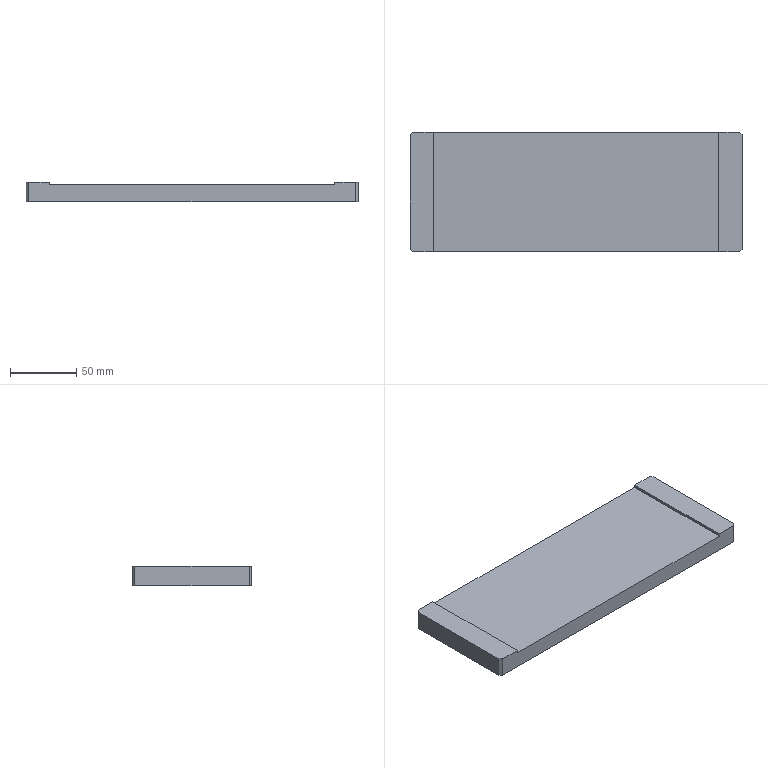Part | STEP file | 001-003-Shaft storage slider connecting plate | 1 solid | 14 faces | box 250 x 90 x 15 mm | volume 298680 mm3 | plane 14
STEP:
#1=CARTESIAN_POINT('',(0.,0.,0.));
#2=DIRECTION('',(0.,0.,1.));
#3=DIRECTION('',(1.,0.,0.));
#4=AXIS2_PLACEMENT_3D('',#1,#2,#3);
#5=CARTESIAN_POINT('',(123.,45.,15.));
#6=VERTEX_POINT('',#5);
#7=CARTESIAN_POINT('',(107.5,45.,15.));
#8=VERTEX_POINT('',#7);
#9=CARTESIAN_POINT('',(-125.,45.,15.));
#10=DIRECTION('',(-1.,0.,0.));
#11=VECTOR('',#10,1.);
#12=LINE('',#9,#11);
#13=CARTESIAN_POINT('',(0.,0.,15.));
#14=DIRECTION('',(0.,0.,-1.));
#15=DIRECTION('',(-1.,0.,0.));
#16=AXIS2_PLACEMENT_3D('',#13,#14,#15);
#17=PLANE('',#16);
#18=CARTESIAN_POINT('',(125.,45.));
#19=DIRECTION('',(1.,0.));
#20=VECTOR('',#19,1.);
#21=LINE('',#18,#20);
#22=(GEOMETRIC_REPRESENTATION_CONTEXT(2)PARAMETRIC_REPRESENTATION_CONTEXT()REPRESENTATION_CONTEXT('',''));
#23=DEFINITIONAL_REPRESENTATION('',(#21),#22);
#24=PCURVE('',#17,#23);
#25=CARTESIAN_POINT('',(-125.,45.,15.));
#26=DIRECTION('',(0.,-1.,0.));
#27=DIRECTION('',(0.,0.,-1.));
#28=AXIS2_PLACEMENT_3D('',#25,#26,#27);
#29=PLANE('',#28);
#30=CARTESIAN_POINT('',(0.,0.));
#31=DIRECTION('',(0.,-1.));
#32=VECTOR('',#31,1.);
#33=LINE('',#30,#32);
#34=(GEOMETRIC_REPRESENTATION_CONTEXT(2)PARAMETRIC_REPRESENTATION_CONTEXT()REPRESENTATION_CONTEXT('',''));
#35=DEFINITIONAL_REPRESENTATION('',(#33),#34);
#36=PCURVE('',#29,#35);
#37=SURFACE_CURVE('',#12,(#24,#36),.PCURVE_S1.);
#38=EDGE_CURVE('',#6,#8,#37,.T.);
#39=ORIENTED_EDGE('',*,*,#38,.T.);
#40=CARTESIAN_POINT('',(107.5,-45.,15.));
#41=VERTEX_POINT('',#40);
#42=CARTESIAN_POINT('',(107.5,-45.,15.));
#43=DIRECTION('',(0.,1.,0.));
#44=VECTOR('',#43,1.);
#45=LINE('',#42,#44);
#46=CARTESIAN_POINT('',(-107.5,-45.));
#47=DIRECTION('',(0.,1.));
#48=VECTOR('',#47,1.);
#49=LINE('',#46,#48);
#50=(GEOMETRIC_REPRESENTATION_CONTEXT(2)PARAMETRIC_REPRESENTATION_CONTEXT()REPRESENTATION_CONTEXT('',''));
#51=DEFINITIONAL_REPRESENTATION('',(#49),#50);
#52=PCURVE('',#17,#51);
#53=CARTESIAN_POINT('',(107.5,-45.,15.));
#54=DIRECTION('',(1.,0.,0.));
#55=DIRECTION('',(0.,0.,-1.));
#56=AXIS2_PLACEMENT_3D('',#53,#54,#55);
#57=PLANE('',#56);
#58=CARTESIAN_POINT('',(0.,0.));
#59=DIRECTION('',(0.,1.));
#60=VECTOR('',#59,1.);
#61=LINE('',#58,#60);
#62=(GEOMETRIC_REPRESENTATION_CONTEXT(2)PARAMETRIC_REPRESENTATION_CONTEXT()REPRESENTATION_CONTEXT('',''));
#63=DEFINITIONAL_REPRESENTATION('',(#61),#62);
#64=PCURVE('',#57,#63);
#65=SURFACE_CURVE('',#45,(#52,#64),.PCURVE_S1.);
#66=EDGE_CURVE('',#41,#8,#65,.T.);
#67=ORIENTED_EDGE('',*,*,#66,.F.);
#68=CARTESIAN_POINT('',(123.,-45.,15.));
#69=VERTEX_POINT('',#68);
#70=CARTESIAN_POINT('',(-125.,-45.,15.));
#71=DIRECTION('',(1.,0.,0.));
#72=VECTOR('',#71,1.);
#73=LINE('',#70,#72);
#74=CARTESIAN_POINT('',(125.,-45.));
#75=DIRECTION('',(-1.,0.));
#76=VECTOR('',#75,1.);
#77=LINE('',#74,#76);
#78=(GEOMETRIC_REPRESENTATION_CONTEXT(2)PARAMETRIC_REPRESENTATION_CONTEXT()REPRESENTATION_CONTEXT('',''));
#79=DEFINITIONAL_REPRESENTATION('',(#77),#78);
#80=PCURVE('',#17,#79);
#81=CARTESIAN_POINT('',(-125.,-45.,15.));
#82=DIRECTION('',(0.,1.,0.));
#83=DIRECTION('',(0.,0.,1.));
#84=AXIS2_PLACEMENT_3D('',#81,#82,#83);
#85=PLANE('',#84);
#86=CARTESIAN_POINT('',(0.,0.));
#87=DIRECTION('',(0.,1.));
#88=VECTOR('',#87,1.);
#89=LINE('',#86,#88);
#90=(GEOMETRIC_REPRESENTATION_CONTEXT(2)PARAMETRIC_REPRESENTATION_CONTEXT()REPRESENTATION_CONTEXT('',''));
#91=DEFINITIONAL_REPRESENTATION('',(#89),#90);
#92=PCURVE('',#85,#91);
#93=SURFACE_CURVE('',#73,(#80,#92),.PCURVE_S1.);
#94=EDGE_CURVE('',#41,#69,#93,.T.);
#95=ORIENTED_EDGE('',*,*,#94,.T.);
#96=CARTESIAN_POINT('',(125.,-43.,15.));
#97=VERTEX_POINT('',#96);
#98=CARTESIAN_POINT('',(125.,-43.,15.));
#99=DIRECTION('',(0.7071,0.7071,0.));
#100=VECTOR('',#99,1.);
#101=LINE('',#98,#100);
#102=CARTESIAN_POINT('',(-125.,-43.));
#103=DIRECTION('',(-0.7071,0.7071));
#104=VECTOR('',#103,1.);
#105=LINE('',#102,#104);
#106=(GEOMETRIC_REPRESENTATION_CONTEXT(2)PARAMETRIC_REPRESENTATION_CONTEXT()REPRESENTATION_CONTEXT('',''));
#107=DEFINITIONAL_REPRESENTATION('',(#105),#106);
#108=PCURVE('',#17,#107);
#109=CARTESIAN_POINT('',(125.,-43.,15.));
#110=DIRECTION('',(-0.7071,0.7071,0.));
#111=DIRECTION('',(0.,0.,-1.));
#112=AXIS2_PLACEMENT_3D('',#109,#110,#111);
#113=PLANE('',#112);
#114=CARTESIAN_POINT('',(0.,0.));
#115=DIRECTION('',(0.,-1.));
#116=VECTOR('',#115,1.);
#117=LINE('',#114,#116);
#118=(GEOMETRIC_REPRESENTATION_CONTEXT(2)PARAMETRIC_REPRESENTATION_CONTEXT()REPRESENTATION_CONTEXT('',''));
#119=DEFINITIONAL_REPRESENTATION('',(#117),#118);
#120=PCURVE('',#113,#119);
#121=SURFACE_CURVE('',#101,(#108,#120),.PCURVE_S1.);
#122=EDGE_CURVE('',#69,#97,#121,.T.);
#123=ORIENTED_EDGE('',*,*,#122,.T.);
#124=CARTESIAN_POINT('',(125.,43.,15.));
#125=VERTEX_POINT('',#124);
#126=CARTESIAN_POINT('',(125.,-45.,15.));
#127=DIRECTION('',(0.,1.,0.));
#128=VECTOR('',#127,1.);
#129=LINE('',#126,#128);
#130=CARTESIAN_POINT('',(-125.,-45.));
#131=DIRECTION('',(0.,1.));
#132=VECTOR('',#131,1.);
#133=LINE('',#130,#132);
#134=(GEOMETRIC_REPRESENTATION_CONTEXT(2)PARAMETRIC_REPRESENTATION_CONTEXT()REPRESENTATION_CONTEXT('',''));
#135=DEFINITIONAL_REPRESENTATION('',(#133),#134);
#136=PCURVE('',#17,#135);
#137=CARTESIAN_POINT('',(125.,-45.,15.));
#138=DIRECTION('',(-1.,0.,0.));
#139=DIRECTION('',(0.,0.,1.));
#140=AXIS2_PLACEMENT_3D('',#137,#138,#139);
#141=PLANE('',#140);
#142=CARTESIAN_POINT('',(0.,0.));
#143=DIRECTION('',(0.,1.));
#144=VECTOR('',#143,1.);
#145=LINE('',#142,#144);
#146=(GEOMETRIC_REPRESENTATION_CONTEXT(2)PARAMETRIC_REPRESENTATION_CONTEXT()REPRESENTATION_CONTEXT('',''));
#147=DEFINITIONAL_REPRESENTATION('',(#145),#146);
#148=PCURVE('',#141,#147);
#149=SURFACE_CURVE('',#129,(#136,#148),.PCURVE_S1.);
#150=EDGE_CURVE('',#97,#125,#149,.T.);
#151=ORIENTED_EDGE('',*,*,#150,.T.);
#152=CARTESIAN_POINT('',(123.,45.,15.));
#153=DIRECTION('',(-0.7071,0.7071,0.));
#154=VECTOR('',#153,1.);
#155=LINE('',#152,#154);
#156=CARTESIAN_POINT('',(-123.,45.));
#157=DIRECTION('',(0.7071,0.7071));
#158=VECTOR('',#157,1.);
#159=LINE('',#156,#158);
#160=(GEOMETRIC_REPRESENTATION_CONTEXT(2)PARAMETRIC_REPRESENTATION_CONTEXT()REPRESENTATION_CONTEXT('',''));
#161=DEFINITIONAL_REPRESENTATION('',(#159),#160);
#162=PCURVE('',#17,#161);
#163=CARTESIAN_POINT('',(123.,45.,15.));
#164=DIRECTION('',(-0.7071,-0.7071,0.));
#165=DIRECTION('',(0.,0.,-1.));
#166=AXIS2_PLACEMENT_3D('',#163,#164,#165);
#167=PLANE('',#166);
#168=CARTESIAN_POINT('',(0.,0.));
#169=DIRECTION('',(0.,-1.));
#170=VECTOR('',#169,1.);
#171=LINE('',#168,#170);
#172=(GEOMETRIC_REPRESENTATION_CONTEXT(2)PARAMETRIC_REPRESENTATION_CONTEXT()REPRESENTATION_CONTEXT('',''));
#173=DEFINITIONAL_REPRESENTATION('',(#171),#172);
#174=PCURVE('',#167,#173);
#175=SURFACE_CURVE('',#155,(#162,#174),.PCURVE_S1.);
#176=EDGE_CURVE('',#125,#6,#175,.T.);
#177=ORIENTED_EDGE('',*,*,#176,.T.);
#178=EDGE_LOOP('',(#39,#67,#95,#123,#151,#177));
#179=FACE_BOUND('',#178,.T.);
#180=ADVANCED_FACE('',(#179),#17,.F.);
#181=ORIENTED_EDGE('',*,*,#150,.F.);
#182=CARTESIAN_POINT('',(125.,-43.,0.));
#183=VERTEX_POINT('',#182);
#184=CARTESIAN_POINT('',(125.,-43.,15.));
#185=DIRECTION('',(0.,0.,-1.));
#186=VECTOR('',#185,1.);
#187=LINE('',#184,#186);
#188=CARTESIAN_POINT('',(0.,2.));
#189=DIRECTION('',(-1.,0.));
#190=VECTOR('',#189,1.);
#191=LINE('',#188,#190);
#192=(GEOMETRIC_REPRESENTATION_CONTEXT(2)PARAMETRIC_REPRESENTATION_CONTEXT()REPRESENTATION_CONTEXT('',''));
#193=DEFINITIONAL_REPRESENTATION('',(#191),#192);
#194=PCURVE('',#141,#193);
#195=CARTESIAN_POINT('',(0.,0.));
#196=DIRECTION('',(1.,0.));
#197=VECTOR('',#196,1.);
#198=LINE('',#195,#197);
#199=(GEOMETRIC_REPRESENTATION_CONTEXT(2)PARAMETRIC_REPRESENTATION_CONTEXT()REPRESENTATION_CONTEXT('',''));
#200=DEFINITIONAL_REPRESENTATION('',(#198),#199);
#201=PCURVE('',#113,#200);
#202=SURFACE_CURVE('',#187,(#194,#201),.PCURVE_S1.);
#203=EDGE_CURVE('',#97,#183,#202,.T.);
#204=ORIENTED_EDGE('',*,*,#203,.T.);
#205=CARTESIAN_POINT('',(125.,43.,0.));
#206=VERTEX_POINT('',#205);
#207=CARTESIAN_POINT('',(125.,-45.,0.));
#208=DIRECTION('',(0.,1.,0.));
#209=VECTOR('',#208,1.);
#210=LINE('',#207,#209);
#211=CARTESIAN_POINT('',(-15.,0.));
#212=DIRECTION('',(0.,1.));
#213=VECTOR('',#212,1.);
#214=LINE('',#211,#213);
#215=(GEOMETRIC_REPRESENTATION_CONTEXT(2)PARAMETRIC_REPRESENTATION_CONTEXT()REPRESENTATION_CONTEXT('',''));
#216=DEFINITIONAL_REPRESENTATION('',(#214),#215);
#217=PCURVE('',#141,#216);
#218=CARTESIAN_POINT('',(0.,0.,0.));
#219=DIRECTION('',(0.,0.,-1.));
#220=DIRECTION('',(-1.,0.,0.));
#221=AXIS2_PLACEMENT_3D('',#218,#219,#220);
#222=PLANE('',#221);
#223=CARTESIAN_POINT('',(-125.,-45.));
#224=DIRECTION('',(0.,1.));
#225=VECTOR('',#224,1.);
#226=LINE('',#223,#225);
#227=(GEOMETRIC_REPRESENTATION_CONTEXT(2)PARAMETRIC_REPRESENTATION_CONTEXT()REPRESENTATION_CONTEXT('',''));
#228=DEFINITIONAL_REPRESENTATION('',(#226),#227);
#229=PCURVE('',#222,#228);
#230=SURFACE_CURVE('',#210,(#217,#229),.PCURVE_S1.);
#231=EDGE_CURVE('',#183,#206,#230,.T.);
#232=ORIENTED_EDGE('',*,*,#231,.T.);
#233=CARTESIAN_POINT('',(125.,43.,15.));
#234=DIRECTION('',(0.,0.,1.));
#235=VECTOR('',#234,1.);
#236=LINE('',#233,#235);
#237=CARTESIAN_POINT('',(0.,88.));
#238=DIRECTION('',(1.,0.));
#239=VECTOR('',#238,1.);
#240=LINE('',#237,#239);
#241=(GEOMETRIC_REPRESENTATION_CONTEXT(2)PARAMETRIC_REPRESENTATION_CONTEXT()REPRESENTATION_CONTEXT('',''));
#242=DEFINITIONAL_REPRESENTATION('',(#240),#241);
#243=PCURVE('',#141,#242);
#244=CARTESIAN_POINT('',(0.,2.828));
#245=DIRECTION('',(-1.,0.));
#246=VECTOR('',#245,1.);
#247=LINE('',#244,#246);
#248=(GEOMETRIC_REPRESENTATION_CONTEXT(2)PARAMETRIC_REPRESENTATION_CONTEXT()REPRESENTATION_CONTEXT('',''));
#249=DEFINITIONAL_REPRESENTATION('',(#247),#248);
#250=PCURVE('',#167,#249);
#251=SURFACE_CURVE('',#236,(#243,#250),.PCURVE_S1.);
#252=EDGE_CURVE('',#206,#125,#251,.T.);
#253=ORIENTED_EDGE('',*,*,#252,.T.);
#254=EDGE_LOOP('',(#181,#204,#232,#253));
#255=FACE_BOUND('',#254,.T.);
#256=ADVANCED_FACE('',(#255),#141,.F.);
#257=CARTESIAN_POINT('',(107.5,45.,13.));
#258=VERTEX_POINT('',#257);
#259=CARTESIAN_POINT('',(-107.5,45.,13.));
#260=VERTEX_POINT('',#259);
#261=CARTESIAN_POINT('',(107.5,45.,13.));
#262=DIRECTION('',(-1.,0.,0.));
#263=VECTOR('',#262,1.);
#264=LINE('',#261,#263);
#265=CARTESIAN_POINT('',(2.,232.5));
#266=DIRECTION('',(0.,-1.));
#267=VECTOR('',#266,1.);
#268=LINE('',#265,#267);
#269=(GEOMETRIC_REPRESENTATION_CONTEXT(2)PARAMETRIC_REPRESENTATION_CONTEXT()REPRESENTATION_CONTEXT('',''));
#270=DEFINITIONAL_REPRESENTATION('',(#268),#269);
#271=PCURVE('',#29,#270);
#272=CARTESIAN_POINT('',(107.5,-45.,13.));
#273=DIRECTION('',(0.,0.,-1.));
#274=DIRECTION('',(-1.,0.,0.));
#275=AXIS2_PLACEMENT_3D('',#272,#273,#274);
#276=PLANE('',#275);
#277=CARTESIAN_POINT('',(0.,90.));
#278=DIRECTION('',(1.,0.));
#279=VECTOR('',#278,1.);
#280=LINE('',#277,#279);
#281=(GEOMETRIC_REPRESENTATION_CONTEXT(2)PARAMETRIC_REPRESENTATION_CONTEXT()REPRESENTATION_CONTEXT('',''));
#282=DEFINITIONAL_REPRESENTATION('',(#280),#281);
#283=PCURVE('',#276,#282);
#284=SURFACE_CURVE('',#264,(#271,#283),.PCURVE_S1.);
#285=EDGE_CURVE('',#258,#260,#284,.T.);
#286=ORIENTED_EDGE('',*,*,#285,.F.);
#287=CARTESIAN_POINT('',(107.5,45.,15.));
#288=DIRECTION('',(0.,0.,-1.));
#289=VECTOR('',#288,1.);
#290=LINE('',#287,#289);
#291=CARTESIAN_POINT('',(0.,232.5));
#292=DIRECTION('',(1.,0.));
#293=VECTOR('',#292,1.);
#294=LINE('',#291,#293);
#295=(GEOMETRIC_REPRESENTATION_CONTEXT(2)PARAMETRIC_REPRESENTATION_CONTEXT()REPRESENTATION_CONTEXT('',''));
#296=DEFINITIONAL_REPRESENTATION('',(#294),#295);
#297=PCURVE('',#29,#296);
#298=CARTESIAN_POINT('',(0.,90.));
#299=DIRECTION('',(1.,0.));
#300=VECTOR('',#299,1.);
#301=LINE('',#298,#300);
#302=(GEOMETRIC_REPRESENTATION_CONTEXT(2)PARAMETRIC_REPRESENTATION_CONTEXT()REPRESENTATION_CONTEXT('',''));
#303=DEFINITIONAL_REPRESENTATION('',(#301),#302);
#304=PCURVE('',#57,#303);
#305=SURFACE_CURVE('',#290,(#297,#304),.PCURVE_S1.);
#306=EDGE_CURVE('',#8,#258,#305,.T.);
#307=ORIENTED_EDGE('',*,*,#306,.F.);
#308=ORIENTED_EDGE('',*,*,#38,.F.);
#309=CARTESIAN_POINT('',(123.,45.,0.));
#310=VERTEX_POINT('',#309);
#311=CARTESIAN_POINT('',(123.,45.,15.));
#312=DIRECTION('',(0.,0.,-1.));
#313=VECTOR('',#312,1.);
#314=LINE('',#311,#313);
#315=CARTESIAN_POINT('',(0.,248.));
#316=DIRECTION('',(1.,0.));
#317=VECTOR('',#316,1.);
#318=LINE('',#315,#317);
#319=(GEOMETRIC_REPRESENTATION_CONTEXT(2)PARAMETRIC_REPRESENTATION_CONTEXT()REPRESENTATION_CONTEXT('',''));
#320=DEFINITIONAL_REPRESENTATION('',(#318),#319);
#321=PCURVE('',#29,#320);
#322=CARTESIAN_POINT('',(0.,0.));
#323=DIRECTION('',(1.,0.));
#324=VECTOR('',#323,1.);
#325=LINE('',#322,#324);
#326=(GEOMETRIC_REPRESENTATION_CONTEXT(2)PARAMETRIC_REPRESENTATION_CONTEXT()REPRESENTATION_CONTEXT('',''));
#327=DEFINITIONAL_REPRESENTATION('',(#325),#326);
#328=PCURVE('',#167,#327);
#329=SURFACE_CURVE('',#314,(#321,#328),.PCURVE_S1.);
#330=EDGE_CURVE('',#6,#310,#329,.T.);
#331=ORIENTED_EDGE('',*,*,#330,.T.);
#332=CARTESIAN_POINT('',(-123.,45.,0.));
#333=VERTEX_POINT('',#332);
#334=CARTESIAN_POINT('',(-125.,45.,0.));
#335=DIRECTION('',(-1.,0.,0.));
#336=VECTOR('',#335,1.);
#337=LINE('',#334,#336);
#338=CARTESIAN_POINT('',(15.,0.));
#339=DIRECTION('',(0.,-1.));
#340=VECTOR('',#339,1.);
#341=LINE('',#338,#340);
#342=(GEOMETRIC_REPRESENTATION_CONTEXT(2)PARAMETRIC_REPRESENTATION_CONTEXT()REPRESENTATION_CONTEXT('',''));
#343=DEFINITIONAL_REPRESENTATION('',(#341),#342);
#344=PCURVE('',#29,#343);
#345=CARTESIAN_POINT('',(125.,45.));
#346=DIRECTION('',(1.,0.));
#347=VECTOR('',#346,1.);
#348=LINE('',#345,#347);
#349=(GEOMETRIC_REPRESENTATION_CONTEXT(2)PARAMETRIC_REPRESENTATION_CONTEXT()REPRESENTATION_CONTEXT('',''));
#350=DEFINITIONAL_REPRESENTATION('',(#348),#349);
#351=PCURVE('',#222,#350);
#352=SURFACE_CURVE('',#337,(#344,#351),.PCURVE_S1.);
#353=EDGE_CURVE('',#310,#333,#352,.T.);
#354=ORIENTED_EDGE('',*,*,#353,.T.);
#355=CARTESIAN_POINT('',(-123.,45.,15.));
#356=VERTEX_POINT('',#355);
#357=CARTESIAN_POINT('',(-123.,45.,15.));
#358=DIRECTION('',(0.,0.,1.));
#359=VECTOR('',#358,1.);
#360=LINE('',#357,#359);
#361=CARTESIAN_POINT('',(0.,2.));
#362=DIRECTION('',(-1.,0.));
#363=VECTOR('',#362,1.);
#364=LINE('',#361,#363);
#365=(GEOMETRIC_REPRESENTATION_CONTEXT(2)PARAMETRIC_REPRESENTATION_CONTEXT()REPRESENTATION_CONTEXT('',''));
#366=DEFINITIONAL_REPRESENTATION('',(#364),#365);
#367=PCURVE('',#29,#366);
#368=CARTESIAN_POINT('',(-125.,43.,15.));
#369=DIRECTION('',(0.7071,-0.7071,0.));
#370=DIRECTION('',(0.,0.,-1.));
#371=AXIS2_PLACEMENT_3D('',#368,#369,#370);
#372=PLANE('',#371);
#373=CARTESIAN_POINT('',(0.,2.828));
#374=DIRECTION('',(-1.,0.));
#375=VECTOR('',#374,1.);
#376=LINE('',#373,#375);
#377=(GEOMETRIC_REPRESENTATION_CONTEXT(2)PARAMETRIC_REPRESENTATION_CONTEXT()REPRESENTATION_CONTEXT('',''));
#378=DEFINITIONAL_REPRESENTATION('',(#376),#377);
#379=PCURVE('',#372,#378);
#380=SURFACE_CURVE('',#360,(#367,#379),.PCURVE_S1.);
#381=EDGE_CURVE('',#333,#356,#380,.T.);
#382=ORIENTED_EDGE('',*,*,#381,.T.);
#383=CARTESIAN_POINT('',(-107.5,45.,15.));
#384=VERTEX_POINT('',#383);
#385=CARTESIAN_POINT('',(-125.,45.,15.));
#386=DIRECTION('',(-1.,0.,0.));
#387=VECTOR('',#386,1.);
#388=LINE('',#385,#387);
#389=CARTESIAN_POINT('',(0.,0.));
#390=DIRECTION('',(0.,-1.));
#391=VECTOR('',#390,1.);
#392=LINE('',#389,#391);
#393=(GEOMETRIC_REPRESENTATION_CONTEXT(2)PARAMETRIC_REPRESENTATION_CONTEXT()REPRESENTATION_CONTEXT('',''));
#394=DEFINITIONAL_REPRESENTATION('',(#392),#393);
#395=PCURVE('',#29,#394);
#396=CARTESIAN_POINT('',(0.,0.,15.));
#397=DIRECTION('',(0.,0.,-1.));
#398=DIRECTION('',(-1.,0.,0.));
#399=AXIS2_PLACEMENT_3D('',#396,#397,#398);
#400=PLANE('',#399);
#401=CARTESIAN_POINT('',(125.,45.));
#402=DIRECTION('',(1.,0.));
#403=VECTOR('',#402,1.);
#404=LINE('',#401,#403);
#405=(GEOMETRIC_REPRESENTATION_CONTEXT(2)PARAMETRIC_REPRESENTATION_CONTEXT()REPRESENTATION_CONTEXT('',''));
#406=DEFINITIONAL_REPRESENTATION('',(#404),#405);
#407=PCURVE('',#400,#406);
#408=SURFACE_CURVE('',#388,(#395,#407),.PCURVE_S1.);
#409=EDGE_CURVE('',#384,#356,#408,.T.);
#410=ORIENTED_EDGE('',*,*,#409,.F.);
#411=CARTESIAN_POINT('',(-107.5,45.,15.));
#412=DIRECTION('',(0.,0.,1.));
#413=VECTOR('',#412,1.);
#414=LINE('',#411,#413);
#415=CARTESIAN_POINT('',(0.,17.5));
#416=DIRECTION('',(-1.,0.));
#417=VECTOR('',#416,1.);
#418=LINE('',#415,#417);
#419=(GEOMETRIC_REPRESENTATION_CONTEXT(2)PARAMETRIC_REPRESENTATION_CONTEXT()REPRESENTATION_CONTEXT('',''));
#420=DEFINITIONAL_REPRESENTATION('',(#418),#419);
#421=PCURVE('',#29,#420);
#422=CARTESIAN_POINT('',(-107.5,-45.,15.));
#423=DIRECTION('',(-1.,0.,0.));
#424=DIRECTION('',(0.,0.,1.));
#425=AXIS2_PLACEMENT_3D('',#422,#423,#424);
#426=PLANE('',#425);
#427=CARTESIAN_POINT('',(0.,90.));
#428=DIRECTION('',(1.,0.));
#429=VECTOR('',#428,1.);
#430=LINE('',#427,#429);
#431=(GEOMETRIC_REPRESENTATION_CONTEXT(2)PARAMETRIC_REPRESENTATION_CONTEXT()REPRESENTATION_CONTEXT('',''));
#432=DEFINITIONAL_REPRESENTATION('',(#430),#431);
#433=PCURVE('',#426,#432);
#434=SURFACE_CURVE('',#414,(#421,#433),.PCURVE_S1.);
#435=EDGE_CURVE('',#260,#384,#434,.T.);
#436=ORIENTED_EDGE('',*,*,#435,.F.);
#437=EDGE_LOOP('',(#286,#307,#308,#331,#354,#382,#410,#436));
#438=FACE_BOUND('',#437,.T.);
#439=ADVANCED_FACE('',(#438),#29,.F.);
#440=CARTESIAN_POINT('',(-125.,43.,0.));
#441=VERTEX_POINT('',#440);
#442=CARTESIAN_POINT('',(-125.,-43.,0.));
#443=VERTEX_POINT('',#442);
#444=CARTESIAN_POINT('',(-125.,-45.,0.));
#445=DIRECTION('',(0.,-1.,0.));
#446=VECTOR('',#445,1.);
#447=LINE('',#444,#446);
#448=CARTESIAN_POINT('',(-125.,-45.,15.));
#449=DIRECTION('',(1.,0.,0.));
#450=DIRECTION('',(0.,0.,-1.));
#451=AXIS2_PLACEMENT_3D('',#448,#449,#450);
#452=PLANE('',#451);
#453=CARTESIAN_POINT('',(15.,0.));
#454=DIRECTION('',(0.,-1.));
#455=VECTOR('',#454,1.);
#456=LINE('',#453,#455);
#457=(GEOMETRIC_REPRESENTATION_CONTEXT(2)PARAMETRIC_REPRESENTATION_CONTEXT()REPRESENTATION_CONTEXT('',''));
#458=DEFINITIONAL_REPRESENTATION('',(#456),#457);
#459=PCURVE('',#452,#458);
#460=CARTESIAN_POINT('',(125.,-45.));
#461=DIRECTION('',(0.,-1.));
#462=VECTOR('',#461,1.);
#463=LINE('',#460,#462);
#464=(GEOMETRIC_REPRESENTATION_CONTEXT(2)PARAMETRIC_REPRESENTATION_CONTEXT()REPRESENTATION_CONTEXT('',''));
#465=DEFINITIONAL_REPRESENTATION('',(#463),#464);
#466=PCURVE('',#222,#465);
#467=SURFACE_CURVE('',#447,(#459,#466),.PCURVE_S1.);
#468=EDGE_CURVE('',#441,#443,#467,.T.);
#469=ORIENTED_EDGE('',*,*,#468,.T.);
#470=CARTESIAN_POINT('',(-125.,-43.,15.));
#471=VERTEX_POINT('',#470);
#472=CARTESIAN_POINT('',(-125.,-43.,15.));
#473=DIRECTION('',(0.,0.,1.));
#474=VECTOR('',#473,1.);
#475=LINE('',#472,#474);
#476=CARTESIAN_POINT('',(0.,2.));
#477=DIRECTION('',(-1.,0.));
#478=VECTOR('',#477,1.);
#479=LINE('',#476,#478);
#480=(GEOMETRIC_REPRESENTATION_CONTEXT(2)PARAMETRIC_REPRESENTATION_CONTEXT()REPRESENTATION_CONTEXT('',''));
#481=DEFINITIONAL_REPRESENTATION('',(#479),#480);
#482=PCURVE('',#452,#481);
#483=CARTESIAN_POINT('',(-123.,-45.,15.));
#484=DIRECTION('',(0.7071,0.7071,0.));
#485=DIRECTION('',(0.,0.,-1.));
#486=AXIS2_PLACEMENT_3D('',#483,#484,#485);
#487=PLANE('',#486);
#488=CARTESIAN_POINT('',(0.,2.828));
#489=DIRECTION('',(-1.,0.));
#490=VECTOR('',#489,1.);
#491=LINE('',#488,#490);
#492=(GEOMETRIC_REPRESENTATION_CONTEXT(2)PARAMETRIC_REPRESENTATION_CONTEXT()REPRESENTATION_CONTEXT('',''));
#493=DEFINITIONAL_REPRESENTATION('',(#491),#492);
#494=PCURVE('',#487,#493);
#495=SURFACE_CURVE('',#475,(#482,#494),.PCURVE_S1.);
#496=EDGE_CURVE('',#443,#471,#495,.T.);
#497=ORIENTED_EDGE('',*,*,#496,.T.);
#498=CARTESIAN_POINT('',(-125.,43.,15.));
#499=VERTEX_POINT('',#498);
#500=CARTESIAN_POINT('',(-125.,-45.,15.));
#501=DIRECTION('',(0.,-1.,0.));
#502=VECTOR('',#501,1.);
#503=LINE('',#500,#502);
#504=CARTESIAN_POINT('',(0.,0.));
#505=DIRECTION('',(0.,-1.));
#506=VECTOR('',#505,1.);
#507=LINE('',#504,#506);
#508=(GEOMETRIC_REPRESENTATION_CONTEXT(2)PARAMETRIC_REPRESENTATION_CONTEXT()REPRESENTATION_CONTEXT('',''));
#509=DEFINITIONAL_REPRESENTATION('',(#507),#508);
#510=PCURVE('',#452,#509);
#511=CARTESIAN_POINT('',(125.,-45.));
#512=DIRECTION('',(0.,-1.));
#513=VECTOR('',#512,1.);
#514=LINE('',#511,#513);
#515=(GEOMETRIC_REPRESENTATION_CONTEXT(2)PARAMETRIC_REPRESENTATION_CONTEXT()REPRESENTATION_CONTEXT('',''));
#516=DEFINITIONAL_REPRESENTATION('',(#514),#515);
#517=PCURVE('',#400,#516);
#518=SURFACE_CURVE('',#503,(#510,#517),.PCURVE_S1.);
#519=EDGE_CURVE('',#499,#471,#518,.T.);
#520=ORIENTED_EDGE('',*,*,#519,.F.);
#521=CARTESIAN_POINT('',(-125.,43.,15.));
#522=DIRECTION('',(0.,0.,-1.));
#523=VECTOR('',#522,1.);
#524=LINE('',#521,#523);
#525=CARTESIAN_POINT('',(0.,88.));
#526=DIRECTION('',(1.,0.));
#527=VECTOR('',#526,1.);
#528=LINE('',#525,#527);
#529=(GEOMETRIC_REPRESENTATION_CONTEXT(2)PARAMETRIC_REPRESENTATION_CONTEXT()REPRESENTATION_CONTEXT('',''));
#530=DEFINITIONAL_REPRESENTATION('',(#528),#529);
#531=PCURVE('',#452,#530);
#532=CARTESIAN_POINT('',(0.,0.));
#533=DIRECTION('',(1.,0.));
#534=VECTOR('',#533,1.);
#535=LINE('',#532,#534);
#536=(GEOMETRIC_REPRESENTATION_CONTEXT(2)PARAMETRIC_REPRESENTATION_CONTEXT()REPRESENTATION_CONTEXT('',''));
#537=DEFINITIONAL_REPRESENTATION('',(#535),#536);
#538=PCURVE('',#372,#537);
#539=SURFACE_CURVE('',#524,(#531,#538),.PCURVE_S1.);
#540=EDGE_CURVE('',#499,#441,#539,.T.);
#541=ORIENTED_EDGE('',*,*,#540,.T.);
#542=EDGE_LOOP('',(#469,#497,#520,#541));
#543=FACE_BOUND('',#542,.T.);
#544=ADVANCED_FACE('',(#543),#452,.F.);
#545=ORIENTED_EDGE('',*,*,#94,.F.);
#546=CARTESIAN_POINT('',(107.5,-45.,13.));
#547=VERTEX_POINT('',#546);
#548=CARTESIAN_POINT('',(107.5,-45.,15.));
#549=DIRECTION('',(0.,0.,-1.));
#550=VECTOR('',#549,1.);
#551=LINE('',#548,#550);
#552=CARTESIAN_POINT('',(0.,232.5));
#553=DIRECTION('',(-1.,0.));
#554=VECTOR('',#553,1.);
#555=LINE('',#552,#554);
#556=(GEOMETRIC_REPRESENTATION_CONTEXT(2)PARAMETRIC_REPRESENTATION_CONTEXT()REPRESENTATION_CONTEXT('',''));
#557=DEFINITIONAL_REPRESENTATION('',(#555),#556);
#558=PCURVE('',#85,#557);
#559=CARTESIAN_POINT('',(0.,0.));
#560=DIRECTION('',(1.,0.));
#561=VECTOR('',#560,1.);
#562=LINE('',#559,#561);
#563=(GEOMETRIC_REPRESENTATION_CONTEXT(2)PARAMETRIC_REPRESENTATION_CONTEXT()REPRESENTATION_CONTEXT('',''));
#564=DEFINITIONAL_REPRESENTATION('',(#562),#563);
#565=PCURVE('',#57,#564);
#566=SURFACE_CURVE('',#551,(#558,#565),.PCURVE_S1.);
#567=EDGE_CURVE('',#41,#547,#566,.T.);
#568=ORIENTED_EDGE('',*,*,#567,.T.);
#569=CARTESIAN_POINT('',(-107.5,-45.,13.));
#570=VERTEX_POINT('',#569);
#571=CARTESIAN_POINT('',(107.5,-45.,13.));
#572=DIRECTION('',(-1.,0.,0.));
#573=VECTOR('',#572,1.);
#574=LINE('',#571,#573);
#575=CARTESIAN_POINT('',(-2.,232.5));
#576=DIRECTION('',(0.,-1.));
#577=VECTOR('',#576,1.);
#578=LINE('',#575,#577);
#579=(GEOMETRIC_REPRESENTATION_CONTEXT(2)PARAMETRIC_REPRESENTATION_CONTEXT()REPRESENTATION_CONTEXT('',''));
#580=DEFINITIONAL_REPRESENTATION('',(#578),#579);
#581=PCURVE('',#85,#580);
#582=CARTESIAN_POINT('',(0.,0.));
#583=DIRECTION('',(1.,0.));
#584=VECTOR('',#583,1.);
#585=LINE('',#582,#584);
#586=(GEOMETRIC_REPRESENTATION_CONTEXT(2)PARAMETRIC_REPRESENTATION_CONTEXT()REPRESENTATION_CONTEXT('',''));
#587=DEFINITIONAL_REPRESENTATION('',(#585),#586);
#588=PCURVE('',#276,#587);
#589=SURFACE_CURVE('',#574,(#581,#588),.PCURVE_S1.);
#590=EDGE_CURVE('',#547,#570,#589,.T.);
#591=ORIENTED_EDGE('',*,*,#590,.T.);
#592=CARTESIAN_POINT('',(-107.5,-45.,15.));
#593=VERTEX_POINT('',#592);
#594=CARTESIAN_POINT('',(-107.5,-45.,15.));
#595=DIRECTION('',(0.,0.,1.));
#596=VECTOR('',#595,1.);
#597=LINE('',#594,#596);
#598=CARTESIAN_POINT('',(0.,17.5));
#599=DIRECTION('',(1.,0.));
#600=VECTOR('',#599,1.);
#601=LINE('',#598,#600);
#602=(GEOMETRIC_REPRESENTATION_CONTEXT(2)PARAMETRIC_REPRESENTATION_CONTEXT()REPRESENTATION_CONTEXT('',''));
#603=DEFINITIONAL_REPRESENTATION('',(#601),#602);
#604=PCURVE('',#85,#603);
#605=CARTESIAN_POINT('',(0.,0.));
#606=DIRECTION('',(1.,0.));
#607=VECTOR('',#606,1.);
#608=LINE('',#605,#607);
#609=(GEOMETRIC_REPRESENTATION_CONTEXT(2)PARAMETRIC_REPRESENTATION_CONTEXT()REPRESENTATION_CONTEXT('',''));
#610=DEFINITIONAL_REPRESENTATION('',(#608),#609);
#611=PCURVE('',#426,#610);
#612=SURFACE_CURVE('',#597,(#604,#611),.PCURVE_S1.);
#613=EDGE_CURVE('',#570,#593,#612,.T.);
#614=ORIENTED_EDGE('',*,*,#613,.T.);
#615=CARTESIAN_POINT('',(-123.,-45.,15.));
#616=VERTEX_POINT('',#615);
#617=CARTESIAN_POINT('',(-125.,-45.,15.));
#618=DIRECTION('',(1.,0.,0.));
#619=VECTOR('',#618,1.);
#620=LINE('',#617,#619);
#621=CARTESIAN_POINT('',(0.,0.));
#622=DIRECTION('',(0.,1.));
#623=VECTOR('',#622,1.);
#624=LINE('',#621,#623);
#625=(GEOMETRIC_REPRESENTATION_CONTEXT(2)PARAMETRIC_REPRESENTATION_CONTEXT()REPRESENTATION_CONTEXT('',''));
#626=DEFINITIONAL_REPRESENTATION('',(#624),#625);
#627=PCURVE('',#85,#626);
#628=CARTESIAN_POINT('',(125.,-45.));
#629=DIRECTION('',(-1.,0.));
#630=VECTOR('',#629,1.);
#631=LINE('',#628,#630);
#632=(GEOMETRIC_REPRESENTATION_CONTEXT(2)PARAMETRIC_REPRESENTATION_CONTEXT()REPRESENTATION_CONTEXT('',''));
#633=DEFINITIONAL_REPRESENTATION('',(#631),#632);
#634=PCURVE('',#400,#633);
#635=SURFACE_CURVE('',#620,(#627,#634),.PCURVE_S1.);
#636=EDGE_CURVE('',#616,#593,#635,.T.);
#637=ORIENTED_EDGE('',*,*,#636,.F.);
#638=CARTESIAN_POINT('',(-123.,-45.,0.));
#639=VERTEX_POINT('',#638);
#640=CARTESIAN_POINT('',(-123.,-45.,15.));
#641=DIRECTION('',(0.,0.,-1.));
#642=VECTOR('',#641,1.);
#643=LINE('',#640,#642);
#644=CARTESIAN_POINT('',(0.,2.));
#645=DIRECTION('',(-1.,0.));
#646=VECTOR('',#645,1.);
#647=LINE('',#644,#646);
#648=(GEOMETRIC_REPRESENTATION_CONTEXT(2)PARAMETRIC_REPRESENTATION_CONTEXT()REPRESENTATION_CONTEXT('',''));
#649=DEFINITIONAL_REPRESENTATION('',(#647),#648);
#650=PCURVE('',#85,#649);
#651=CARTESIAN_POINT('',(0.,0.));
#652=DIRECTION('',(1.,0.));
#653=VECTOR('',#652,1.);
#654=LINE('',#651,#653);
#655=(GEOMETRIC_REPRESENTATION_CONTEXT(2)PARAMETRIC_REPRESENTATION_CONTEXT()REPRESENTATION_CONTEXT('',''));
#656=DEFINITIONAL_REPRESENTATION('',(#654),#655);
#657=PCURVE('',#487,#656);
#658=SURFACE_CURVE('',#643,(#650,#657),.PCURVE_S1.);
#659=EDGE_CURVE('',#616,#639,#658,.T.);
#660=ORIENTED_EDGE('',*,*,#659,.T.);
#661=CARTESIAN_POINT('',(123.,-45.,0.));
#662=VERTEX_POINT('',#661);
#663=CARTESIAN_POINT('',(-125.,-45.,0.));
#664=DIRECTION('',(1.,0.,0.));
#665=VECTOR('',#664,1.);
#666=LINE('',#663,#665);
#667=CARTESIAN_POINT('',(-15.,0.));
#668=DIRECTION('',(0.,1.));
#669=VECTOR('',#668,1.);
#670=LINE('',#667,#669);
#671=(GEOMETRIC_REPRESENTATION_CONTEXT(2)PARAMETRIC_REPRESENTATION_CONTEXT()REPRESENTATION_CONTEXT('',''));
#672=DEFINITIONAL_REPRESENTATION('',(#670),#671);
#673=PCURVE('',#85,#672);
#674=CARTESIAN_POINT('',(125.,-45.));
#675=DIRECTION('',(-1.,0.));
#676=VECTOR('',#675,1.);
#677=LINE('',#674,#676);
#678=(GEOMETRIC_REPRESENTATION_CONTEXT(2)PARAMETRIC_REPRESENTATION_CONTEXT()REPRESENTATION_CONTEXT('',''));
#679=DEFINITIONAL_REPRESENTATION('',(#677),#678);
#680=PCURVE('',#222,#679);
#681=SURFACE_CURVE('',#666,(#673,#680),.PCURVE_S1.);
#682=EDGE_CURVE('',#639,#662,#681,.T.);
#683=ORIENTED_EDGE('',*,*,#682,.T.);
#684=CARTESIAN_POINT('',(123.,-45.,15.));
#685=DIRECTION('',(0.,0.,1.));
#686=VECTOR('',#685,1.);
#687=LINE('',#684,#686);
#688=CARTESIAN_POINT('',(0.,248.));
#689=DIRECTION('',(1.,0.));
#690=VECTOR('',#689,1.);
#691=LINE('',#688,#690);
#692=(GEOMETRIC_REPRESENTATION_CONTEXT(2)PARAMETRIC_REPRESENTATION_CONTEXT()REPRESENTATION_CONTEXT('',''));
#693=DEFINITIONAL_REPRESENTATION('',(#691),#692);
#694=PCURVE('',#85,#693);
#695=CARTESIAN_POINT('',(0.,2.828));
#696=DIRECTION('',(-1.,0.));
#697=VECTOR('',#696,1.);
#698=LINE('',#695,#697);
#699=(GEOMETRIC_REPRESENTATION_CONTEXT(2)PARAMETRIC_REPRESENTATION_CONTEXT()REPRESENTATION_CONTEXT('',''));
#700=DEFINITIONAL_REPRESENTATION('',(#698),#699);
#701=PCURVE('',#113,#700);
#702=SURFACE_CURVE('',#687,(#694,#701),.PCURVE_S1.);
#703=EDGE_CURVE('',#662,#69,#702,.T.);
#704=ORIENTED_EDGE('',*,*,#703,.T.);
#705=EDGE_LOOP('',(#545,#568,#591,#614,#637,#660,#683,#704));
#706=FACE_BOUND('',#705,.T.);
#707=ADVANCED_FACE('',(#706),#85,.F.);
#708=ORIENTED_EDGE('',*,*,#636,.T.);
#709=CARTESIAN_POINT('',(-107.5,-45.,15.));
#710=DIRECTION('',(0.,1.,0.));
#711=VECTOR('',#710,1.);
#712=LINE('',#709,#711);
#713=CARTESIAN_POINT('',(107.5,-45.));
#714=DIRECTION('',(0.,1.));
#715=VECTOR('',#714,1.);
#716=LINE('',#713,#715);
#717=(GEOMETRIC_REPRESENTATION_CONTEXT(2)PARAMETRIC_REPRESENTATION_CONTEXT()REPRESENTATION_CONTEXT('',''));
#718=DEFINITIONAL_REPRESENTATION('',(#716),#717);
#719=PCURVE('',#400,#718);
#720=CARTESIAN_POINT('',(0.,0.));
#721=DIRECTION('',(0.,1.));
#722=VECTOR('',#721,1.);
#723=LINE('',#720,#722);
#724=(GEOMETRIC_REPRESENTATION_CONTEXT(2)PARAMETRIC_REPRESENTATION_CONTEXT()REPRESENTATION_CONTEXT('',''));
#725=DEFINITIONAL_REPRESENTATION('',(#723),#724);
#726=PCURVE('',#426,#725);
#727=SURFACE_CURVE('',#712,(#719,#726),.PCURVE_S1.);
#728=EDGE_CURVE('',#593,#384,#727,.T.);
#729=ORIENTED_EDGE('',*,*,#728,.T.);
#730=ORIENTED_EDGE('',*,*,#409,.T.);
#731=CARTESIAN_POINT('',(-125.,43.,15.));
#732=DIRECTION('',(-0.7071,-0.7071,0.));
#733=VECTOR('',#732,1.);
#734=LINE('',#731,#733);
#735=CARTESIAN_POINT('',(125.,43.));
#736=DIRECTION('',(0.7071,-0.7071));
#737=VECTOR('',#736,1.);
#738=LINE('',#735,#737);
#739=(GEOMETRIC_REPRESENTATION_CONTEXT(2)PARAMETRIC_REPRESENTATION_CONTEXT()REPRESENTATION_CONTEXT('',''));
#740=DEFINITIONAL_REPRESENTATION('',(#738),#739);
#741=PCURVE('',#400,#740);
#742=CARTESIAN_POINT('',(0.,0.));
#743=DIRECTION('',(0.,-1.));
#744=VECTOR('',#743,1.);
#745=LINE('',#742,#744);
#746=(GEOMETRIC_REPRESENTATION_CONTEXT(2)PARAMETRIC_REPRESENTATION_CONTEXT()REPRESENTATION_CONTEXT('',''));
#747=DEFINITIONAL_REPRESENTATION('',(#745),#746);
#748=PCURVE('',#372,#747);
#749=SURFACE_CURVE('',#734,(#741,#748),.PCURVE_S1.);
#750=EDGE_CURVE('',#356,#499,#749,.T.);
#751=ORIENTED_EDGE('',*,*,#750,.T.);
#752=ORIENTED_EDGE('',*,*,#519,.T.);
#753=CARTESIAN_POINT('',(-123.,-45.,15.));
#754=DIRECTION('',(0.7071,-0.7071,0.));
#755=VECTOR('',#754,1.);
#756=LINE('',#753,#755);
#757=CARTESIAN_POINT('',(123.,-45.));
#758=DIRECTION('',(-0.7071,-0.7071));
#759=VECTOR('',#758,1.);
#760=LINE('',#757,#759);
#761=(GEOMETRIC_REPRESENTATION_CONTEXT(2)PARAMETRIC_REPRESENTATION_CONTEXT()REPRESENTATION_CONTEXT('',''));
#762=DEFINITIONAL_REPRESENTATION('',(#760),#761);
#763=PCURVE('',#400,#762);
#764=CARTESIAN_POINT('',(0.,0.));
#765=DIRECTION('',(0.,-1.));
#766=VECTOR('',#765,1.);
#767=LINE('',#764,#766);
#768=(GEOMETRIC_REPRESENTATION_CONTEXT(2)PARAMETRIC_REPRESENTATION_CONTEXT()REPRESENTATION_CONTEXT('',''));
#769=DEFINITIONAL_REPRESENTATION('',(#767),#768);
#770=PCURVE('',#487,#769);
#771=SURFACE_CURVE('',#756,(#763,#770),.PCURVE_S1.);
#772=EDGE_CURVE('',#471,#616,#771,.T.);
#773=ORIENTED_EDGE('',*,*,#772,.T.);
#774=EDGE_LOOP('',(#708,#729,#730,#751,#752,#773));
#775=FACE_BOUND('',#774,.T.);
#776=ADVANCED_FACE('',(#775),#400,.F.);
#777=ORIENTED_EDGE('',*,*,#231,.F.);
#778=CARTESIAN_POINT('',(84.,-84.,0.));
#779=DIRECTION('',(-0.7071,-0.7071,0.));
#780=VECTOR('',#779,1.);
#781=LINE('',#778,#780);
#782=CARTESIAN_POINT('',(-84.,-84.));
#783=DIRECTION('',(0.7071,-0.7071));
#784=VECTOR('',#783,1.);
#785=LINE('',#782,#784);
#786=(GEOMETRIC_REPRESENTATION_CONTEXT(2)PARAMETRIC_REPRESENTATION_CONTEXT()REPRESENTATION_CONTEXT('',''));
#787=DEFINITIONAL_REPRESENTATION('',(#785),#786);
#788=PCURVE('',#222,#787);
#789=CARTESIAN_POINT('',(15.,57.983));
#790=DIRECTION('',(0.,1.));
#791=VECTOR('',#790,1.);
#792=LINE('',#789,#791);
#793=(GEOMETRIC_REPRESENTATION_CONTEXT(2)PARAMETRIC_REPRESENTATION_CONTEXT()REPRESENTATION_CONTEXT('',''));
#794=DEFINITIONAL_REPRESENTATION('',(#792),#793);
#795=PCURVE('',#113,#794);
#796=SURFACE_CURVE('',#781,(#788,#795),.PCURVE_S1.);
#797=EDGE_CURVE('',#183,#662,#796,.T.);
#798=ORIENTED_EDGE('',*,*,#797,.T.);
#799=ORIENTED_EDGE('',*,*,#682,.F.);
#800=CARTESIAN_POINT('',(-84.,-84.,0.));
#801=DIRECTION('',(-0.7071,0.7071,0.));
#802=VECTOR('',#801,1.);
#803=LINE('',#800,#802);
#804=CARTESIAN_POINT('',(84.,-84.));
#805=DIRECTION('',(0.7071,0.7071));
#806=VECTOR('',#805,1.);
#807=LINE('',#804,#806);
#808=(GEOMETRIC_REPRESENTATION_CONTEXT(2)PARAMETRIC_REPRESENTATION_CONTEXT()REPRESENTATION_CONTEXT('',''));
#809=DEFINITIONAL_REPRESENTATION('',(#807),#808);
#810=PCURVE('',#222,#809);
#811=CARTESIAN_POINT('',(15.,-55.154));
#812=DIRECTION('',(0.,1.));
#813=VECTOR('',#812,1.);
#814=LINE('',#811,#813);
#815=(GEOMETRIC_REPRESENTATION_CONTEXT(2)PARAMETRIC_REPRESENTATION_CONTEXT()REPRESENTATION_CONTEXT('',''));
#816=DEFINITIONAL_REPRESENTATION('',(#814),#815);
#817=PCURVE('',#487,#816);
#818=SURFACE_CURVE('',#803,(#810,#817),.PCURVE_S1.);
#819=EDGE_CURVE('',#639,#443,#818,.T.);
#820=ORIENTED_EDGE('',*,*,#819,.T.);
#821=ORIENTED_EDGE('',*,*,#468,.F.);
#822=CARTESIAN_POINT('',(-84.,84.,0.));
#823=DIRECTION('',(0.7071,0.7071,0.));
#824=VECTOR('',#823,1.);
#825=LINE('',#822,#824);
#826=CARTESIAN_POINT('',(84.,84.));
#827=DIRECTION('',(-0.7071,0.7071));
#828=VECTOR('',#827,1.);
#829=LINE('',#826,#828);
#830=(GEOMETRIC_REPRESENTATION_CONTEXT(2)PARAMETRIC_REPRESENTATION_CONTEXT()REPRESENTATION_CONTEXT('',''));
#831=DEFINITIONAL_REPRESENTATION('',(#829),#830);
#832=PCURVE('',#222,#831);
#833=CARTESIAN_POINT('',(15.,57.983));
#834=DIRECTION('',(0.,1.));
#835=VECTOR('',#834,1.);
#836=LINE('',#833,#835);
#837=(GEOMETRIC_REPRESENTATION_CONTEXT(2)PARAMETRIC_REPRESENTATION_CONTEXT()REPRESENTATION_CONTEXT('',''));
#838=DEFINITIONAL_REPRESENTATION('',(#836),#837);
#839=PCURVE('',#372,#838);
#840=SURFACE_CURVE('',#825,(#832,#839),.PCURVE_S1.);
#841=EDGE_CURVE('',#441,#333,#840,.T.);
#842=ORIENTED_EDGE('',*,*,#841,.T.);
#843=ORIENTED_EDGE('',*,*,#353,.F.);
#844=CARTESIAN_POINT('',(84.,84.,0.));
#845=DIRECTION('',(0.7071,-0.7071,0.));
#846=VECTOR('',#845,1.);
#847=LINE('',#844,#846);
#848=CARTESIAN_POINT('',(-84.,84.));
#849=DIRECTION('',(-0.7071,-0.7071));
#850=VECTOR('',#849,1.);
#851=LINE('',#848,#850);
#852=(GEOMETRIC_REPRESENTATION_CONTEXT(2)PARAMETRIC_REPRESENTATION_CONTEXT()REPRESENTATION_CONTEXT('',''));
#853=DEFINITIONAL_REPRESENTATION('',(#851),#852);
#854=PCURVE('',#222,#853);
#855=CARTESIAN_POINT('',(15.,-55.154));
#856=DIRECTION('',(0.,1.));
#857=VECTOR('',#856,1.);
#858=LINE('',#855,#857);
#859=(GEOMETRIC_REPRESENTATION_CONTEXT(2)PARAMETRIC_REPRESENTATION_CONTEXT()REPRESENTATION_CONTEXT('',''));
#860=DEFINITIONAL_REPRESENTATION('',(#858),#859);
#861=PCURVE('',#167,#860);
#862=SURFACE_CURVE('',#847,(#854,#861),.PCURVE_S1.);
#863=EDGE_CURVE('',#310,#206,#862,.T.);
#864=ORIENTED_EDGE('',*,*,#863,.T.);
#865=EDGE_LOOP('',(#777,#798,#799,#820,#821,#842,#843,#864));
#866=FACE_BOUND('',#865,.T.);
#867=ADVANCED_FACE('',(#866),#222,.T.);
#868=ORIENTED_EDGE('',*,*,#122,.F.);
#869=ORIENTED_EDGE('',*,*,#703,.F.);
#870=ORIENTED_EDGE('',*,*,#797,.F.);
#871=ORIENTED_EDGE('',*,*,#203,.F.);
#872=EDGE_LOOP('',(#868,#869,#870,#871));
#873=FACE_BOUND('',#872,.T.);
#874=ADVANCED_FACE('',(#873),#113,.F.);
#875=ORIENTED_EDGE('',*,*,#772,.F.);
#876=ORIENTED_EDGE('',*,*,#496,.F.);
#877=ORIENTED_EDGE('',*,*,#819,.F.);
#878=ORIENTED_EDGE('',*,*,#659,.F.);
#879=EDGE_LOOP('',(#875,#876,#877,#878));
#880=FACE_BOUND('',#879,.T.);
#881=ADVANCED_FACE('',(#880),#487,.F.);
#882=ORIENTED_EDGE('',*,*,#750,.F.);
#883=ORIENTED_EDGE('',*,*,#381,.F.);
#884=ORIENTED_EDGE('',*,*,#841,.F.);
#885=ORIENTED_EDGE('',*,*,#540,.F.);
#886=EDGE_LOOP('',(#882,#883,#884,#885));
#887=FACE_BOUND('',#886,.T.);
#888=ADVANCED_FACE('',(#887),#372,.F.);
#889=ORIENTED_EDGE('',*,*,#176,.F.);
#890=ORIENTED_EDGE('',*,*,#252,.F.);
#891=ORIENTED_EDGE('',*,*,#863,.F.);
#892=ORIENTED_EDGE('',*,*,#330,.F.);
#893=EDGE_LOOP('',(#889,#890,#891,#892));
#894=FACE_BOUND('',#893,.T.);
#895=ADVANCED_FACE('',(#894),#167,.F.);
#896=ORIENTED_EDGE('',*,*,#306,.T.);
#897=CARTESIAN_POINT('',(107.5,-45.,13.));
#898=DIRECTION('',(0.,1.,0.));
#899=VECTOR('',#898,1.);
#900=LINE('',#897,#899);
#901=CARTESIAN_POINT('',(2.,0.));
#902=DIRECTION('',(0.,1.));
#903=VECTOR('',#902,1.);
#904=LINE('',#901,#903);
#905=(GEOMETRIC_REPRESENTATION_CONTEXT(2)PARAMETRIC_REPRESENTATION_CONTEXT()REPRESENTATION_CONTEXT('',''));
#906=DEFINITIONAL_REPRESENTATION('',(#904),#905);
#907=PCURVE('',#57,#906);
#908=CARTESIAN_POINT('',(0.,0.));
#909=DIRECTION('',(0.,1.));
#910=VECTOR('',#909,1.);
#911=LINE('',#908,#910);
#912=(GEOMETRIC_REPRESENTATION_CONTEXT(2)PARAMETRIC_REPRESENTATION_CONTEXT()REPRESENTATION_CONTEXT('',''));
#913=DEFINITIONAL_REPRESENTATION('',(#911),#912);
#914=PCURVE('',#276,#913);
#915=SURFACE_CURVE('',#900,(#907,#914),.PCURVE_S1.);
#916=EDGE_CURVE('',#547,#258,#915,.T.);
#917=ORIENTED_EDGE('',*,*,#916,.F.);
#918=ORIENTED_EDGE('',*,*,#567,.F.);
#919=ORIENTED_EDGE('',*,*,#66,.T.);
#920=EDGE_LOOP('',(#896,#917,#918,#919));
#921=FACE_BOUND('',#920,.T.);
#922=ADVANCED_FACE('',(#921),#57,.F.);
#923=ORIENTED_EDGE('',*,*,#435,.T.);
#924=ORIENTED_EDGE('',*,*,#728,.F.);
#925=ORIENTED_EDGE('',*,*,#613,.F.);
#926=CARTESIAN_POINT('',(-107.5,-45.,13.));
#927=DIRECTION('',(0.,1.,0.));
#928=VECTOR('',#927,1.);
#929=LINE('',#926,#928);
#930=CARTESIAN_POINT('',(-2.,0.));
#931=DIRECTION('',(0.,1.));
#932=VECTOR('',#931,1.);
#933=LINE('',#930,#932);
#934=(GEOMETRIC_REPRESENTATION_CONTEXT(2)PARAMETRIC_REPRESENTATION_CONTEXT()REPRESENTATION_CONTEXT('',''));
#935=DEFINITIONAL_REPRESENTATION('',(#933),#934);
#936=PCURVE('',#426,#935);
#937=CARTESIAN_POINT('',(215.,0.));
#938=DIRECTION('',(0.,1.));
#939=VECTOR('',#938,1.);
#940=LINE('',#937,#939);
#941=(GEOMETRIC_REPRESENTATION_CONTEXT(2)PARAMETRIC_REPRESENTATION_CONTEXT()REPRESENTATION_CONTEXT('',''));
#942=DEFINITIONAL_REPRESENTATION('',(#940),#941);
#943=PCURVE('',#276,#942);
#944=SURFACE_CURVE('',#929,(#936,#943),.PCURVE_S1.);
#945=EDGE_CURVE('',#570,#260,#944,.T.);
#946=ORIENTED_EDGE('',*,*,#945,.T.);
#947=EDGE_LOOP('',(#923,#924,#925,#946));
#948=FACE_BOUND('',#947,.T.);
#949=ADVANCED_FACE('',(#948),#426,.F.);
#950=ORIENTED_EDGE('',*,*,#285,.T.);
#951=ORIENTED_EDGE('',*,*,#945,.F.);
#952=ORIENTED_EDGE('',*,*,#590,.F.);
#953=ORIENTED_EDGE('',*,*,#916,.T.);
#954=EDGE_LOOP('',(#950,#951,#952,#953));
#955=FACE_BOUND('',#954,.T.);
#956=ADVANCED_FACE('',(#955),#276,.F.);
#957=CLOSED_SHELL('',(#180,#256,#439,#544,#707,#776,#867,#874,#881,#888,#895,#922,#949,#956));
#958=MANIFOLD_SOLID_BREP('',#957);
#959=(LENGTH_UNIT()NAMED_UNIT(*)SI_UNIT(.MILLI.,.METRE.));
#960=UNCERTAINTY_MEASURE_WITH_UNIT(LENGTH_MEASURE(0.0000001),#959,'','');
#961=(NAMED_UNIT(*)PLANE_ANGLE_UNIT()SI_UNIT($,.RADIAN.));
#962=(NAMED_UNIT(*)SI_UNIT($,.STERADIAN.)SOLID_ANGLE_UNIT());
#963=(GEOMETRIC_REPRESENTATION_CONTEXT(3)GLOBAL_UNCERTAINTY_ASSIGNED_CONTEXT((#960))GLOBAL_UNIT_ASSIGNED_CONTEXT((#959,#961,#962))REPRESENTATION_CONTEXT('',''));
#964=ADVANCED_BREP_SHAPE_REPRESENTATION('',(#4,#958),#963);